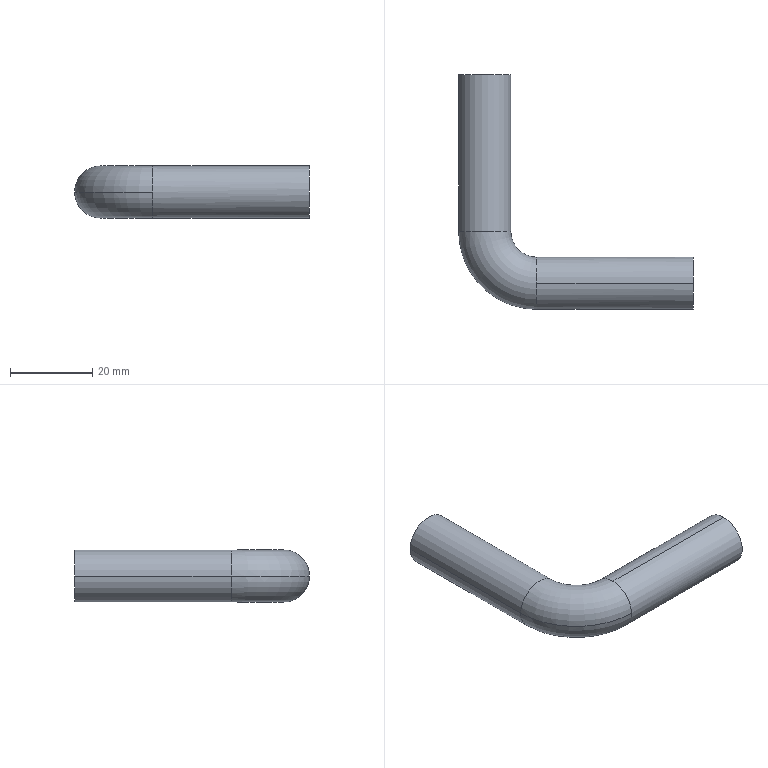Part | SolidWorks | features 3DProfileFeature 1, Sweep 1 | 1 solid | 8 faces | box 57.15 x 57.15 x 12.7 mm | volume 12180 mm3 | cylinder 4 | torus 2 | plane 2 | commonest cylinder face diameters 12.7 x4
STEP:
#1=CARTESIAN_POINT('',(-42.394,-24.239,-6.35));
#2=VERTEX_POINT('',#1);
#3=CARTESIAN_POINT('',(-42.394,-30.589,0.));
#4=VERTEX_POINT('',#3);
#5=CARTESIAN_POINT('',(-42.394,-24.239,0.));
#6=DIRECTION('',(-1.,0.,0.));
#7=DIRECTION('',(0.,0.,1.));
#8=AXIS2_PLACEMENT_3D('',#5,#6,#7);
#9=CIRCLE('',#8,6.35);
#10=EDGE_CURVE('',#2,#4,#9,.T.);
#11=ORIENTED_EDGE('',*,*,#10,.T.);
#12=CARTESIAN_POINT('',(-61.444,-11.539,0.));
#13=VERTEX_POINT('',#12);
#14=CARTESIAN_POINT('',(-42.394,-11.539,0.));
#15=DIRECTION('',(0.,0.,-1.));
#16=DIRECTION('',(-1.,0.,0.));
#17=AXIS2_PLACEMENT_3D('',#14,#15,#16);
#18=CIRCLE('',#17,19.05);
#19=EDGE_CURVE('',#4,#13,#18,.T.);
#20=ORIENTED_EDGE('',*,*,#19,.T.);
#21=CARTESIAN_POINT('',(-48.744,-11.539,0.));
#22=VERTEX_POINT('',#21);
#23=CARTESIAN_POINT('',(-55.094,-11.539,0.));
#24=DIRECTION('',(0.,1.,0.));
#25=DIRECTION('',(0.,0.,1.));
#26=AXIS2_PLACEMENT_3D('',#23,#24,#25);
#27=CIRCLE('',#26,6.35);
#28=EDGE_CURVE('',#22,#13,#27,.T.);
#29=ORIENTED_EDGE('',*,*,#28,.F.);
#30=CARTESIAN_POINT('',(-42.394,-17.889,0.));
#31=VERTEX_POINT('',#30);
#32=CARTESIAN_POINT('',(-42.394,-11.539,0.));
#33=DIRECTION('',(0.,0.,-1.));
#34=DIRECTION('',(-1.,0.,0.));
#35=AXIS2_PLACEMENT_3D('',#32,#33,#34);
#36=CIRCLE('',#35,6.35);
#37=EDGE_CURVE('',#31,#22,#36,.T.);
#38=ORIENTED_EDGE('',*,*,#37,.F.);
#39=CARTESIAN_POINT('',(-42.394,-24.239,0.));
#40=DIRECTION('',(-1.,0.,0.));
#41=DIRECTION('',(0.,0.,1.));
#42=AXIS2_PLACEMENT_3D('',#39,#40,#41);
#43=CIRCLE('',#42,6.35);
#44=EDGE_CURVE('',#31,#2,#43,.T.);
#45=ORIENTED_EDGE('',*,*,#44,.T.);
#46=EDGE_LOOP('',(#11,#20,#29,#38,#45));
#47=FACE_OUTER_BOUND('',#46,.T.);
#48=CARTESIAN_POINT('',(-42.394,-11.539,0.));
#49=DIRECTION('',(0.,0.,-1.));
#50=DIRECTION('',(-1.,0.,0.));
#51=AXIS2_PLACEMENT_3D('',#48,#49,#50);
#52=TOROIDAL_SURFACE('',#51,12.7,6.35);
#53=ADVANCED_FACE('',(#47),#52,.T.);
#54=CARTESIAN_POINT('',(-42.394,-24.239,6.35));
#55=VERTEX_POINT('',#54);
#56=CARTESIAN_POINT('',(-42.394,-24.239,0.));
#57=DIRECTION('',(-1.,0.,0.));
#58=DIRECTION('',(0.,0.,1.));
#59=AXIS2_PLACEMENT_3D('',#56,#57,#58);
#60=CIRCLE('',#59,6.35);
#61=EDGE_CURVE('',#55,#31,#60,.T.);
#62=ORIENTED_EDGE('',*,*,#61,.F.);
#63=CARTESIAN_POINT('',(-4.294,-24.239,6.35));
#64=VERTEX_POINT('',#63);
#65=CARTESIAN_POINT('',(-42.394,-24.239,6.35));
#66=DIRECTION('',(1.,0.,0.));
#67=VECTOR('',#66,1000.);
#68=LINE('',#65,#67);
#69=EDGE_CURVE('',#55,#64,#68,.T.);
#70=ORIENTED_EDGE('',*,*,#69,.T.);
#71=CARTESIAN_POINT('',(-4.294,-24.239,-6.35));
#72=VERTEX_POINT('',#71);
#73=CARTESIAN_POINT('',(-4.294,-24.239,0.));
#74=DIRECTION('',(-1.,0.,0.));
#75=DIRECTION('',(0.,0.,1.));
#76=AXIS2_PLACEMENT_3D('',#73,#74,#75);
#77=CIRCLE('',#76,6.35);
#78=EDGE_CURVE('',#64,#72,#77,.T.);
#79=ORIENTED_EDGE('',*,*,#78,.T.);
#80=CARTESIAN_POINT('',(-42.394,-24.239,-6.35));
#81=DIRECTION('',(1.,0.,0.));
#82=VECTOR('',#81,1000.);
#83=LINE('',#80,#82);
#84=EDGE_CURVE('',#2,#72,#83,.T.);
#85=ORIENTED_EDGE('',*,*,#84,.F.);
#86=ORIENTED_EDGE('',*,*,#44,.F.);
#87=EDGE_LOOP('',(#62,#70,#79,#85,#86));
#88=FACE_OUTER_BOUND('',#87,.T.);
#89=CARTESIAN_POINT('',(-42.394,-24.239,0.));
#90=DIRECTION('',(1.,0.,0.));
#91=DIRECTION('',(0.,0.,-1.));
#92=AXIS2_PLACEMENT_3D('',#89,#90,#91);
#93=CYLINDRICAL_SURFACE('',#92,6.35);
#94=ADVANCED_FACE('',(#88),#93,.T.);
#95=CARTESIAN_POINT('',(-55.094,-11.539,0.));
#96=DIRECTION('',(0.,1.,0.));
#97=DIRECTION('',(0.,0.,1.));
#98=AXIS2_PLACEMENT_3D('',#95,#96,#97);
#99=CIRCLE('',#98,6.35);
#100=EDGE_CURVE('',#13,#22,#99,.T.);
#101=ORIENTED_EDGE('',*,*,#100,.T.);
#102=CARTESIAN_POINT('',(-48.744,26.561,0.));
#103=VERTEX_POINT('',#102);
#104=CARTESIAN_POINT('',(-48.744,-11.539,0.));
#105=DIRECTION('',(0.,1.,0.));
#106=VECTOR('',#105,1000.);
#107=LINE('',#104,#106);
#108=EDGE_CURVE('',#22,#103,#107,.T.);
#109=ORIENTED_EDGE('',*,*,#108,.T.);
#110=CARTESIAN_POINT('',(-61.444,26.561,0.));
#111=VERTEX_POINT('',#110);
#112=CARTESIAN_POINT('',(-55.094,26.561,0.));
#113=DIRECTION('',(0.,1.,0.));
#114=DIRECTION('',(0.,0.,1.));
#115=AXIS2_PLACEMENT_3D('',#112,#113,#114);
#116=CIRCLE('',#115,6.35);
#117=EDGE_CURVE('',#111,#103,#116,.T.);
#118=ORIENTED_EDGE('',*,*,#117,.F.);
#119=CARTESIAN_POINT('',(-61.444,-11.539,0.));
#120=DIRECTION('',(0.,1.,0.));
#121=VECTOR('',#120,1000.);
#122=LINE('',#119,#121);
#123=EDGE_CURVE('',#13,#111,#122,.T.);
#124=ORIENTED_EDGE('',*,*,#123,.F.);
#125=EDGE_LOOP('',(#101,#109,#118,#124));
#126=FACE_OUTER_BOUND('',#125,.T.);
#127=CARTESIAN_POINT('',(-55.094,-11.539,0.));
#128=DIRECTION('',(0.,1.,0.));
#129=DIRECTION('',(-1.,0.,0.));
#130=AXIS2_PLACEMENT_3D('',#127,#128,#129);
#131=CYLINDRICAL_SURFACE('',#130,6.35);
#132=ADVANCED_FACE('',(#126),#131,.T.);
#133=ORIENTED_EDGE('',*,*,#108,.F.);
#134=ORIENTED_EDGE('',*,*,#28,.T.);
#135=ORIENTED_EDGE('',*,*,#123,.T.);
#136=CARTESIAN_POINT('',(-55.094,26.561,0.));
#137=DIRECTION('',(0.,1.,0.));
#138=DIRECTION('',(0.,0.,1.));
#139=AXIS2_PLACEMENT_3D('',#136,#137,#138);
#140=CIRCLE('',#139,6.35);
#141=EDGE_CURVE('',#103,#111,#140,.T.);
#142=ORIENTED_EDGE('',*,*,#141,.F.);
#143=EDGE_LOOP('',(#133,#134,#135,#142));
#144=FACE_OUTER_BOUND('',#143,.T.);
#145=CARTESIAN_POINT('',(-55.094,-11.539,0.));
#146=DIRECTION('',(0.,1.,0.));
#147=DIRECTION('',(-1.,0.,0.));
#148=AXIS2_PLACEMENT_3D('',#145,#146,#147);
#149=CYLINDRICAL_SURFACE('',#148,6.35);
#150=ADVANCED_FACE('',(#144),#149,.T.);
#151=ORIENTED_EDGE('',*,*,#19,.F.);
#152=CARTESIAN_POINT('',(-42.394,-24.239,0.));
#153=DIRECTION('',(-1.,0.,0.));
#154=DIRECTION('',(0.,0.,1.));
#155=AXIS2_PLACEMENT_3D('',#152,#153,#154);
#156=CIRCLE('',#155,6.35);
#157=EDGE_CURVE('',#4,#55,#156,.T.);
#158=ORIENTED_EDGE('',*,*,#157,.T.);
#159=ORIENTED_EDGE('',*,*,#61,.T.);
#160=ORIENTED_EDGE('',*,*,#37,.T.);
#161=ORIENTED_EDGE('',*,*,#100,.F.);
#162=EDGE_LOOP('',(#151,#158,#159,#160,#161));
#163=FACE_OUTER_BOUND('',#162,.T.);
#164=CARTESIAN_POINT('',(-42.394,-11.539,0.));
#165=DIRECTION('',(0.,0.,-1.));
#166=DIRECTION('',(-1.,0.,0.));
#167=AXIS2_PLACEMENT_3D('',#164,#165,#166);
#168=TOROIDAL_SURFACE('',#167,12.7,6.35);
#169=ADVANCED_FACE('',(#163),#168,.T.);
#170=ORIENTED_EDGE('',*,*,#69,.F.);
#171=ORIENTED_EDGE('',*,*,#157,.F.);
#172=ORIENTED_EDGE('',*,*,#10,.F.);
#173=ORIENTED_EDGE('',*,*,#84,.T.);
#174=CARTESIAN_POINT('',(-4.294,-24.239,0.));
#175=DIRECTION('',(-1.,0.,0.));
#176=DIRECTION('',(0.,0.,1.));
#177=AXIS2_PLACEMENT_3D('',#174,#175,#176);
#178=CIRCLE('',#177,6.35);
#179=EDGE_CURVE('',#72,#64,#178,.T.);
#180=ORIENTED_EDGE('',*,*,#179,.T.);
#181=EDGE_LOOP('',(#170,#171,#172,#173,#180));
#182=FACE_OUTER_BOUND('',#181,.T.);
#183=CARTESIAN_POINT('',(-42.394,-24.239,0.));
#184=DIRECTION('',(1.,0.,0.));
#185=DIRECTION('',(0.,0.,-1.));
#186=AXIS2_PLACEMENT_3D('',#183,#184,#185);
#187=CYLINDRICAL_SURFACE('',#186,6.35);
#188=ADVANCED_FACE('',(#182),#187,.T.);
#189=ORIENTED_EDGE('',*,*,#117,.T.);
#190=ORIENTED_EDGE('',*,*,#141,.T.);
#191=EDGE_LOOP('',(#189,#190));
#192=FACE_OUTER_BOUND('',#191,.T.);
#193=CARTESIAN_POINT('',(-55.094,26.561,0.));
#194=DIRECTION('',(0.,1.,0.));
#195=DIRECTION('',(0.,0.,1.));
#196=AXIS2_PLACEMENT_3D('',#193,#194,#195);
#197=PLANE('',#196);
#198=ADVANCED_FACE('',(#192),#197,.T.);
#199=ORIENTED_EDGE('',*,*,#179,.F.);
#200=ORIENTED_EDGE('',*,*,#78,.F.);
#201=EDGE_LOOP('',(#199,#200));
#202=FACE_OUTER_BOUND('',#201,.T.);
#203=CARTESIAN_POINT('',(-4.294,-24.239,0.));
#204=DIRECTION('',(-1.,0.,0.));
#205=DIRECTION('',(0.,0.,1.));
#206=AXIS2_PLACEMENT_3D('',#203,#204,#205);
#207=PLANE('',#206);
#208=ADVANCED_FACE('',(#202),#207,.F.);
#209=CLOSED_SHELL('',(#53,#94,#132,#150,#169,#188,#198,#208));
#210=MANIFOLD_SOLID_BREP('',#209);
#211=CARTESIAN_POINT('',(0.,0.,0.));
#212=DIRECTION('',(0.,0.,1.));
#213=DIRECTION('',(1.,0.,0.));
#214=AXIS2_PLACEMENT_3D('',#211,#212,#213);
#215=(LENGTH_UNIT()NAMED_UNIT(*)SI_UNIT(.MILLI.,.METRE.));
#216=UNCERTAINTY_MEASURE_WITH_UNIT(LENGTH_MEASURE(0.00001),#215,'','');
#217=(NAMED_UNIT(*)PLANE_ANGLE_UNIT()SI_UNIT($,.RADIAN.));
#218=(NAMED_UNIT(*)SI_UNIT($,.STERADIAN.)SOLID_ANGLE_UNIT());
#219=(GEOMETRIC_REPRESENTATION_CONTEXT(3)GLOBAL_UNCERTAINTY_ASSIGNED_CONTEXT((#216))GLOBAL_UNIT_ASSIGNED_CONTEXT((#215,#217,#218))REPRESENTATION_CONTEXT('',''));
#220=ADVANCED_BREP_SHAPE_REPRESENTATION('',(#210,#214),#219);